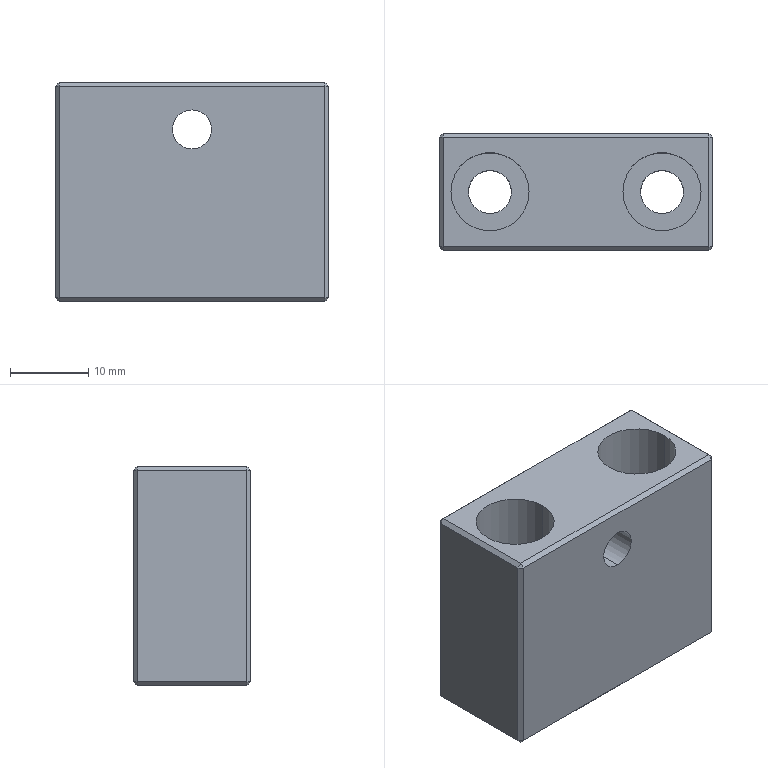Part | STEP file | ND25021-01-JDKM-10-TL | 1 solid | 38 faces | box 35 x 15 x 28 mm | volume 12116 mm3 | plane 28 | cylinder 10 | commonest cylinder face diameters 5.5 x4 10 x4 5 x2